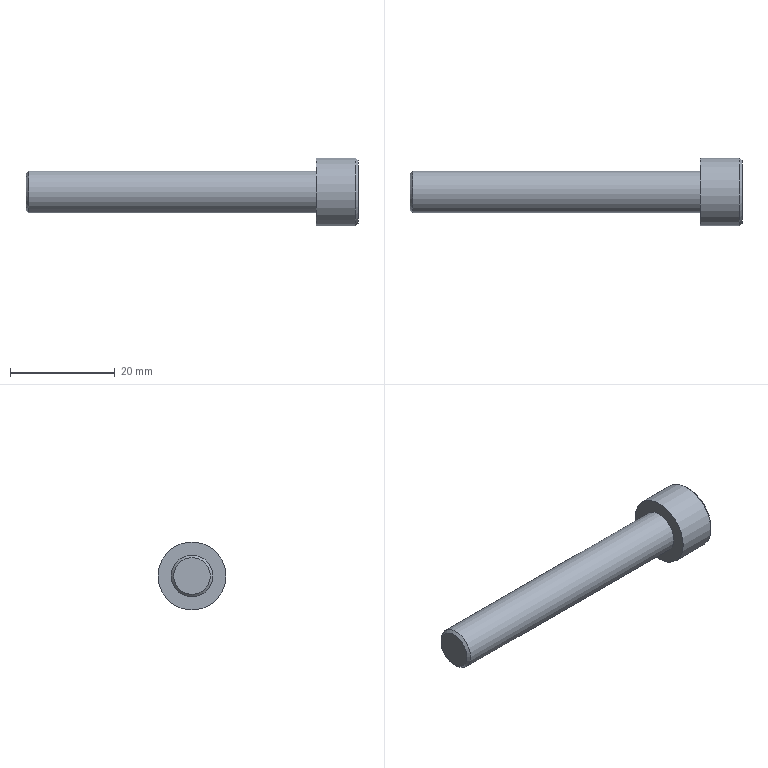Part | NX | features CHAMFER 6, BREP 2, solid 2, SUBTRACT 1 | 1 solid | 36 faces | box 63.5 x 13 x 13 mm | volume 3707 mm3 | plane 23 | spline 9 | cylinder 2 | cone 2 | commonest cylinder face diameters 8 x1 13 x1
STEP:
#1=CARTESIAN_POINT('',(272.5,-202.45,31.002));
#2=VERTEX_POINT('',#1);
#3=CARTESIAN_POINT('',(272.5,-202.625,31.545));
#4=VERTEX_POINT('',#3);
#5=CARTESIAN_POINT('',(272.5,-202.45,31.002));
#6=CARTESIAN_POINT('',(272.5,-202.385,31.002));
#7=CARTESIAN_POINT('',(272.5,-202.327,31.016));
#8=CARTESIAN_POINT('',(272.5,-202.225,31.073));
#9=CARTESIAN_POINT('',(272.5,-202.185,31.113));
#10=CARTESIAN_POINT('',(272.5,-202.128,31.215));
#11=CARTESIAN_POINT('',(272.5,-202.114,31.272));
#12=CARTESIAN_POINT('',(272.5,-202.114,31.377));
#13=CARTESIAN_POINT('',(272.5,-202.121,31.418));
#14=CARTESIAN_POINT('',(272.5,-202.15,31.497));
#15=CARTESIAN_POINT('',(272.5,-202.171,31.531));
#16=CARTESIAN_POINT('',(272.5,-202.224,31.589));
#17=CARTESIAN_POINT('',(272.5,-202.256,31.611));
#18=CARTESIAN_POINT('',(272.5,-202.327,31.643));
#19=CARTESIAN_POINT('',(272.5,-202.366,31.651));
#20=CARTESIAN_POINT('',(272.5,-202.452,31.651));
#21=CARTESIAN_POINT('',(272.5,-202.491,31.642));
#22=CARTESIAN_POINT('',(272.5,-202.562,31.608));
#23=CARTESIAN_POINT('',(272.5,-202.595,31.581));
#24=CARTESIAN_POINT('',(272.5,-202.625,31.545));
#25=B_SPLINE_CURVE_WITH_KNOTS('',3,(#5,#6,#7,#8,#9,#10,#11,#12,#13,#14,#15,#16,#17,#18,#19,#20,#21,#22,#23,#24),.UNSPECIFIED.,.F.,.F.,(4,2,2,2,2,2,2,2,2,4),(0.,0.02844,0.05688,0.08532,0.1049,0.1245,0.144,0.1636,0.184,0.2044),.UNSPECIFIED.);
#26=EDGE_CURVE('',#2,#4,#25,.T.);
#27=ORIENTED_EDGE('',*,*,#26,.F.);
#28=CARTESIAN_POINT('',(272.5,-202.314,31.783));
#29=VERTEX_POINT('',#28);
#30=CARTESIAN_POINT('',(272.5,-202.314,31.783));
#31=CARTESIAN_POINT('',(272.5,-202.306,31.762));
#32=CARTESIAN_POINT('',(272.5,-202.294,31.746));
#33=CARTESIAN_POINT('',(272.5,-202.262,31.722));
#34=CARTESIAN_POINT('',(272.5,-202.245,31.716));
#35=CARTESIAN_POINT('',(272.5,-202.205,31.716));
#36=CARTESIAN_POINT('',(272.5,-202.188,31.724));
#37=CARTESIAN_POINT('',(272.5,-202.16,31.754));
#38=CARTESIAN_POINT('',(272.5,-202.154,31.77));
#39=CARTESIAN_POINT('',(272.5,-202.154,31.818));
#40=CARTESIAN_POINT('',(272.5,-202.164,31.85));
#41=CARTESIAN_POINT('',(272.5,-202.208,31.915));
#42=CARTESIAN_POINT('',(272.5,-202.241,31.943));
#43=CARTESIAN_POINT('',(272.5,-202.327,31.987));
#44=CARTESIAN_POINT('',(272.5,-202.377,31.998));
#45=CARTESIAN_POINT('',(272.5,-202.493,31.998));
#46=CARTESIAN_POINT('',(272.5,-202.545,31.987));
#47=CARTESIAN_POINT('',(272.5,-202.637,31.943));
#48=CARTESIAN_POINT('',(272.5,-202.676,31.91));
#49=CARTESIAN_POINT('',(272.5,-202.741,31.823));
#50=CARTESIAN_POINT('',(272.5,-202.766,31.769));
#51=CARTESIAN_POINT('',(272.5,-202.8,31.637));
#52=CARTESIAN_POINT('',(272.5,-202.809,31.562));
#53=CARTESIAN_POINT('',(272.5,-202.809,31.375));
#54=CARTESIAN_POINT('',(272.5,-202.795,31.288));
#55=CARTESIAN_POINT('',(272.5,-202.738,31.146));
#56=CARTESIAN_POINT('',(272.5,-202.696,31.093));
#57=CARTESIAN_POINT('',(272.5,-202.588,31.02));
#58=CARTESIAN_POINT('',(272.5,-202.524,31.002));
#59=CARTESIAN_POINT('',(272.5,-202.45,31.002));
#60=B_SPLINE_CURVE_WITH_KNOTS('',3,(#30,#31,#32,#33,#34,#35,#36,#37,#38,#39,#40,#41,#42,#43,#44,#45,#46,#47,#48,#49,#50,#51,#52,#53,#54,#55,#56,#57,#58,#59),.UNSPECIFIED.,.F.,.F.,(4,2,2,2,2,2,2,2,2,2,2,2,2,2,4),(0.3727,0.3977,0.4227,0.4513,0.4798,0.5272,0.5745,0.6219,0.6711,0.7203,0.7695,0.8188,0.8792,0.9396,1.),.UNSPECIFIED.);
#61=EDGE_CURVE('',#29,#2,#60,.T.);
#62=ORIENTED_EDGE('',*,*,#61,.F.);
#63=CARTESIAN_POINT('',(272.5,-202.568,31.796));
#64=VERTEX_POINT('',#63);
#65=CARTESIAN_POINT('',(272.5,-202.568,31.796));
#66=CARTESIAN_POINT('',(272.5,-202.552,31.819));
#67=CARTESIAN_POINT('',(272.5,-202.532,31.837));
#68=CARTESIAN_POINT('',(272.5,-202.486,31.864));
#69=CARTESIAN_POINT('',(272.5,-202.463,31.871));
#70=CARTESIAN_POINT('',(272.5,-202.41,31.871));
#71=CARTESIAN_POINT('',(272.5,-202.384,31.863));
#72=CARTESIAN_POINT('',(272.5,-202.34,31.831));
#73=CARTESIAN_POINT('',(272.5,-202.324,31.809));
#74=CARTESIAN_POINT('',(272.5,-202.314,31.783));
#75=B_SPLINE_CURVE_WITH_KNOTS('',3,(#65,#66,#67,#68,#69,#70,#71,#72,#73,#74),.UNSPECIFIED.,.F.,.F.,(4,2,2,2,4),(0.2569,0.2827,0.3085,0.3406,0.3727),.UNSPECIFIED.);
#76=EDGE_CURVE('',#64,#29,#75,.T.);
#77=ORIENTED_EDGE('',*,*,#76,.F.);
#78=CARTESIAN_POINT('',(272.5,-202.625,31.545));
#79=CARTESIAN_POINT('',(272.5,-202.619,31.666));
#80=CARTESIAN_POINT('',(272.5,-202.6,31.749));
#81=CARTESIAN_POINT('',(272.5,-202.568,31.796));
#82=B_SPLINE_CURVE_WITH_KNOTS('',3,(#78,#79,#80,#81),.UNSPECIFIED.,.F.,.F.,(4,4),(0.2044,0.2569),.PIECEWISE_BEZIER_KNOTS.);
#83=EDGE_CURVE('',#4,#64,#82,.T.);
#84=ORIENTED_EDGE('',*,*,#83,.F.);
#85=EDGE_LOOP('',(#27,#62,#77,#84));
#86=FACE_BOUND('',#85,.T.);
#87=CARTESIAN_POINT('',(272.5,-204.732,28.5));
#88=VERTEX_POINT('',#87);
#89=CARTESIAN_POINT('',(272.5,-206.464,31.5));
#90=VERTEX_POINT('',#89);
#91=CARTESIAN_POINT('',(272.5,-206.464,31.5));
#92=DIRECTION('',(0.,-0.5,0.866));
#93=VECTOR('',#92,1000.);
#94=LINE('',#91,#93);
#95=EDGE_CURVE('',#88,#90,#94,.T.);
#96=ORIENTED_EDGE('',*,*,#95,.F.);
#97=CARTESIAN_POINT('',(272.5,-201.268,28.5));
#98=VERTEX_POINT('',#97);
#99=CARTESIAN_POINT('',(272.5,-204.732,28.5));
#100=DIRECTION('',(0.,-1.,0.));
#101=VECTOR('',#100,1000.);
#102=LINE('',#99,#101);
#103=EDGE_CURVE('',#98,#88,#102,.T.);
#104=ORIENTED_EDGE('',*,*,#103,.F.);
#105=CARTESIAN_POINT('',(272.5,-199.536,31.5));
#106=VERTEX_POINT('',#105);
#107=CARTESIAN_POINT('',(272.5,-201.268,28.5));
#108=DIRECTION('',(0.,-0.5,-0.866));
#109=VECTOR('',#108,1000.);
#110=LINE('',#107,#109);
#111=EDGE_CURVE('',#106,#98,#110,.T.);
#112=ORIENTED_EDGE('',*,*,#111,.F.);
#113=CARTESIAN_POINT('',(272.5,-201.268,34.5));
#114=VERTEX_POINT('',#113);
#115=CARTESIAN_POINT('',(272.5,-199.536,31.5));
#116=DIRECTION('',(0.,0.5,-0.866));
#117=VECTOR('',#116,1000.);
#118=LINE('',#115,#117);
#119=EDGE_CURVE('',#114,#106,#118,.T.);
#120=ORIENTED_EDGE('',*,*,#119,.F.);
#121=CARTESIAN_POINT('',(272.5,-204.732,34.5));
#122=VERTEX_POINT('',#121);
#123=CARTESIAN_POINT('',(272.5,-201.268,34.5));
#124=DIRECTION('',(0.,1.,0.));
#125=VECTOR('',#124,1000.);
#126=LINE('',#123,#125);
#127=EDGE_CURVE('',#122,#114,#126,.T.);
#128=ORIENTED_EDGE('',*,*,#127,.F.);
#129=CARTESIAN_POINT('',(272.5,-204.732,34.5));
#130=DIRECTION('',(0.,0.5,0.866));
#131=VECTOR('',#130,1000.);
#132=LINE('',#129,#131);
#133=EDGE_CURVE('',#90,#122,#132,.T.);
#134=ORIENTED_EDGE('',*,*,#133,.F.);
#135=EDGE_LOOP('',(#96,#104,#112,#120,#128,#134));
#136=FACE_BOUND('',#135,.T.);
#137=CARTESIAN_POINT('',(272.5,-203.797,31.005));
#138=VERTEX_POINT('',#137);
#139=CARTESIAN_POINT('',(272.5,-203.706,31.783));
#140=VERTEX_POINT('',#139);
#141=CARTESIAN_POINT('',(272.5,-203.797,31.005));
#142=CARTESIAN_POINT('',(272.5,-203.769,31.005));
#143=CARTESIAN_POINT('',(272.5,-203.748,31.014));
#144=CARTESIAN_POINT('',(272.5,-203.715,31.051));
#145=CARTESIAN_POINT('',(272.5,-203.706,31.079));
#146=CARTESIAN_POINT('',(272.5,-203.706,31.338));
#147=CARTESIAN_POINT('',(272.5,-203.706,31.561));
#148=CARTESIAN_POINT('',(272.5,-203.706,31.783));
#149=B_SPLINE_CURVE_WITH_KNOTS('',3,(#141,#142,#143,#144,#145,#146,#147,#148),.UNSPECIFIED.,.F.,.F.,(4,2,2,4),(0.,0.01767,0.03533,0.1418),.UNSPECIFIED.);
#150=EDGE_CURVE('',#138,#140,#149,.T.);
#151=ORIENTED_EDGE('',*,*,#150,.F.);
#152=CARTESIAN_POINT('',(272.5,-203.561,31.859));
#153=VERTEX_POINT('',#152);
#154=CARTESIAN_POINT('',(272.5,-203.561,31.859));
#155=CARTESIAN_POINT('',(272.5,-203.571,31.898));
#156=CARTESIAN_POINT('',(272.5,-203.58,31.925));
#157=CARTESIAN_POINT('',(272.5,-203.596,31.96));
#158=CARTESIAN_POINT('',(272.5,-203.608,31.972));
#159=CARTESIAN_POINT('',(272.5,-203.641,31.985));
#160=CARTESIAN_POINT('',(272.5,-203.667,31.988));
#161=CARTESIAN_POINT('',(272.5,-203.724,31.988));
#162=CARTESIAN_POINT('',(272.5,-203.744,31.988));
#163=CARTESIAN_POINT('',(272.5,-203.802,31.988));
#164=CARTESIAN_POINT('',(272.5,-203.831,31.981));
#165=CARTESIAN_POINT('',(272.5,-203.875,31.951));
#166=CARTESIAN_POINT('',(272.5,-203.886,31.923));
#167=CARTESIAN_POINT('',(272.5,-203.886,31.626));
#168=CARTESIAN_POINT('',(272.5,-203.886,31.371));
#169=CARTESIAN_POINT('',(272.5,-203.886,31.079));
#170=CARTESIAN_POINT('',(272.5,-203.878,31.051));
#171=CARTESIAN_POINT('',(272.5,-203.845,31.014));
#172=CARTESIAN_POINT('',(272.5,-203.823,31.005));
#173=CARTESIAN_POINT('',(272.5,-203.797,31.005));
#174=B_SPLINE_CURVE_WITH_KNOTS('',3,(#154,#155,#156,#157,#158,#159,#160,#161,#162,#163,#164,#165,#166,#167,#168,#169,#170,#171,#172,#173),.UNSPECIFIED.,.F.,.F.,(4,2,2,2,2,2,2,2,2,4),(0.8075,0.8217,0.8358,0.85,0.8578,0.8723,0.8868,0.9743,0.9872,1.),.UNSPECIFIED.);
#175=EDGE_CURVE('',#153,#138,#174,.T.);
#176=ORIENTED_EDGE('',*,*,#175,.F.);
#177=CARTESIAN_POINT('',(272.5,-203.42,31.33));
#178=VERTEX_POINT('',#177);
#179=CARTESIAN_POINT('',(272.5,-203.435,31.385));
#180=DIRECTION('',(0.,-0.2564,0.9666));
#181=VECTOR('',#180,1000.);
#182=LINE('',#179,#181);
#183=EDGE_CURVE('',#178,#153,#182,.T.);
#184=ORIENTED_EDGE('',*,*,#183,.F.);
#185=CARTESIAN_POINT('',(272.5,-203.28,31.859));
#186=VERTEX_POINT('',#185);
#187=CARTESIAN_POINT('',(272.5,-203.35,31.593));
#188=DIRECTION('',(0.,-0.2564,-0.9666));
#189=VECTOR('',#188,1000.);
#190=LINE('',#187,#189);
#191=EDGE_CURVE('',#186,#178,#190,.T.);
#192=ORIENTED_EDGE('',*,*,#191,.F.);
#193=CARTESIAN_POINT('',(272.5,-203.134,31.783));
#194=VERTEX_POINT('',#193);
#195=CARTESIAN_POINT('',(272.5,-203.134,31.783));
#196=CARTESIAN_POINT('',(272.5,-203.134,31.561));
#197=CARTESIAN_POINT('',(272.5,-203.134,31.338));
#198=CARTESIAN_POINT('',(272.5,-203.134,31.079));
#199=CARTESIAN_POINT('',(272.5,-203.126,31.051));
#200=CARTESIAN_POINT('',(272.5,-203.092,31.014));
#201=CARTESIAN_POINT('',(272.5,-203.071,31.005));
#202=CARTESIAN_POINT('',(272.5,-203.018,31.005));
#203=CARTESIAN_POINT('',(272.5,-202.995,31.014));
#204=CARTESIAN_POINT('',(272.5,-202.962,31.051));
#205=CARTESIAN_POINT('',(272.5,-202.954,31.079));
#206=CARTESIAN_POINT('',(272.5,-202.954,31.371));
#207=CARTESIAN_POINT('',(272.5,-202.954,31.626));
#208=CARTESIAN_POINT('',(272.5,-202.954,31.923));
#209=CARTESIAN_POINT('',(272.5,-202.965,31.951));
#210=CARTESIAN_POINT('',(272.5,-203.009,31.981));
#211=CARTESIAN_POINT('',(272.5,-203.039,31.988));
#212=CARTESIAN_POINT('',(272.5,-203.096,31.988));
#213=CARTESIAN_POINT('',(272.5,-203.117,31.988));
#214=CARTESIAN_POINT('',(272.5,-203.173,31.988));
#215=CARTESIAN_POINT('',(272.5,-203.2,31.985));
#216=CARTESIAN_POINT('',(272.5,-203.233,31.972));
#217=CARTESIAN_POINT('',(272.5,-203.245,31.96));
#218=CARTESIAN_POINT('',(272.5,-203.261,31.925));
#219=CARTESIAN_POINT('',(272.5,-203.27,31.898));
#220=CARTESIAN_POINT('',(272.5,-203.28,31.859));
#221=B_SPLINE_CURVE_WITH_KNOTS('',3,(#195,#196,#197,#198,#199,#200,#201,#202,#203,#204,#205,#206,#207,#208,#209,#210,#211,#212,#213,#214,#215,#216,#217,#218,#219,#220),.UNSPECIFIED.,.F.,.F.,(4,2,2,2,2,2,2,2,2,2,2,2,4),(0.3909,0.4624,0.4743,0.4862,0.4988,0.5115,0.599,0.6135,0.628,0.6359,0.65,0.6642,0.6783),.UNSPECIFIED.);
#222=EDGE_CURVE('',#194,#186,#221,.T.);
#223=ORIENTED_EDGE('',*,*,#222,.F.);
#224=CARTESIAN_POINT('',(272.5,-203.289,31.167));
#225=VERTEX_POINT('',#224);
#226=CARTESIAN_POINT('',(272.5,-203.193,31.549));
#227=DIRECTION('',(0.,0.244,0.9698));
#228=VECTOR('',#227,1000.);
#229=LINE('',#226,#228);
#230=EDGE_CURVE('',#225,#194,#229,.T.);
#231=ORIENTED_EDGE('',*,*,#230,.F.);
#232=CARTESIAN_POINT('',(272.5,-203.551,31.167));
#233=VERTEX_POINT('',#232);
#234=CARTESIAN_POINT('',(272.5,-203.551,31.167));
#235=CARTESIAN_POINT('',(272.5,-203.546,31.147));
#236=CARTESIAN_POINT('',(272.5,-203.541,31.128));
#237=CARTESIAN_POINT('',(272.5,-203.531,31.09));
#238=CARTESIAN_POINT('',(272.5,-203.524,31.073));
#239=CARTESIAN_POINT('',(272.5,-203.506,31.043));
#240=CARTESIAN_POINT('',(272.5,-203.494,31.03));
#241=CARTESIAN_POINT('',(272.5,-203.462,31.01));
#242=CARTESIAN_POINT('',(272.5,-203.443,31.005));
#243=CARTESIAN_POINT('',(272.5,-203.39,31.005));
#244=CARTESIAN_POINT('',(272.5,-203.366,31.013));
#245=CARTESIAN_POINT('',(272.5,-203.332,31.044));
#246=CARTESIAN_POINT('',(272.5,-203.32,31.061));
#247=CARTESIAN_POINT('',(272.5,-203.307,31.098));
#248=CARTESIAN_POINT('',(272.5,-203.299,31.127));
#249=CARTESIAN_POINT('',(272.5,-203.289,31.167));
#250=B_SPLINE_CURVE_WITH_KNOTS('',3,(#234,#235,#236,#237,#238,#239,#240,#241,#242,#243,#244,#245,#246,#247,#248,#249),.UNSPECIFIED.,.F.,.F.,(4,2,2,2,2,2,2,4),(0.243,0.253,0.263,0.273,0.283,0.2963,0.3096,0.3228),.UNSPECIFIED.);
#251=EDGE_CURVE('',#233,#225,#250,.T.);
#252=ORIENTED_EDGE('',*,*,#251,.F.);
#253=CARTESIAN_POINT('',(272.5,-203.597,31.35));
#254=DIRECTION('',(0.,0.244,-0.9698));
#255=VECTOR('',#254,1000.);
#256=LINE('',#253,#255);
#257=EDGE_CURVE('',#140,#233,#256,.T.);
#258=ORIENTED_EDGE('',*,*,#257,.F.);
#259=EDGE_LOOP('',(#151,#176,#184,#192,#223,#231,#252,#258));
#260=FACE_BOUND('',#259,.T.);
#261=CARTESIAN_POINT('',(272.5,-203.,31.5));
#262=DIRECTION('',(1.,0.,0.));
#263=DIRECTION('',(0.,-1.,0.));
#264=AXIS2_PLACEMENT_3D('',#261,#262,#263);
#265=PLANE('',#264);
#266=ADVANCED_FACE('',(#86,#136,#260),#265,.T.);
#267=CARTESIAN_POINT('',(213.,-206.5,31.5));
#268=VERTEX_POINT('',#267);
#269=CARTESIAN_POINT('',(213.,-203.,31.5));
#270=DIRECTION('',(-1.,0.,0.));
#271=DIRECTION('',(0.,-1.,0.));
#272=AXIS2_PLACEMENT_3D('',#269,#270,#271);
#273=CIRCLE('',#272,3.5);
#274=EDGE_CURVE('',#268,#268,#273,.T.);
#275=ORIENTED_EDGE('',*,*,#274,.T.);
#276=EDGE_LOOP('',(#275));
#277=FACE_BOUND('',#276,.T.);
#278=CARTESIAN_POINT('',(213.,-203.,27.5));
#279=DIRECTION('',(-1.,0.,0.));
#280=DIRECTION('',(0.,1.,0.));
#281=AXIS2_PLACEMENT_3D('',#278,#279,#280);
#282=PLANE('',#281);
#283=ADVANCED_FACE('',(#277),#282,.T.);
#284=CARTESIAN_POINT('',(213.5,-207.,31.5));
#285=VERTEX_POINT('',#284);
#286=CARTESIAN_POINT('',(213.5,-203.,31.5));
#287=DIRECTION('',(1.,0.,0.));
#288=DIRECTION('',(0.,-1.,0.));
#289=AXIS2_PLACEMENT_3D('',#286,#287,#288);
#290=CIRCLE('',#289,4.);
#291=EDGE_CURVE('',#285,#285,#290,.T.);
#292=ORIENTED_EDGE('',*,*,#291,.T.);
#293=EDGE_LOOP('',(#292));
#294=FACE_BOUND('',#293,.T.);
#295=CARTESIAN_POINT('',(268.5,-199.,31.5));
#296=VERTEX_POINT('',#295);
#297=CARTESIAN_POINT('',(268.5,-203.,31.5));
#298=DIRECTION('',(1.,0.,0.));
#299=DIRECTION('',(0.,1.,0.));
#300=AXIS2_PLACEMENT_3D('',#297,#298,#299);
#301=CIRCLE('',#300,4.);
#302=EDGE_CURVE('',#296,#296,#301,.T.);
#303=ORIENTED_EDGE('',*,*,#302,.F.);
#304=EDGE_LOOP('',(#303));
#305=FACE_BOUND('',#304,.T.);
#306=CARTESIAN_POINT('',(277.5,-203.,31.5));
#307=DIRECTION('',(1.,0.,0.));
#308=DIRECTION('',(0.,-1.,0.));
#309=AXIS2_PLACEMENT_3D('',#306,#307,#308);
#310=CYLINDRICAL_SURFACE('',#309,4.);
#311=ADVANCED_FACE('',(#294,#305),#310,.T.);
#312=ORIENTED_EDGE('',*,*,#302,.T.);
#313=EDGE_LOOP('',(#312));
#314=FACE_BOUND('',#313,.T.);
#315=CARTESIAN_POINT('',(268.5,-196.5,31.5));
#316=VERTEX_POINT('',#315);
#317=CARTESIAN_POINT('',(268.5,-203.,31.5));
#318=DIRECTION('',(1.,0.,0.));
#319=DIRECTION('',(0.,1.,0.));
#320=AXIS2_PLACEMENT_3D('',#317,#318,#319);
#321=CIRCLE('',#320,6.5);
#322=EDGE_CURVE('',#316,#316,#321,.T.);
#323=ORIENTED_EDGE('',*,*,#322,.F.);
#324=EDGE_LOOP('',(#323));
#325=FACE_BOUND('',#324,.T.);
#326=CARTESIAN_POINT('',(268.5,-203.,25.));
#327=DIRECTION('',(-1.,0.,0.));
#328=DIRECTION('',(0.,1.,0.));
#329=AXIS2_PLACEMENT_3D('',#326,#327,#328);
#330=PLANE('',#329);
#331=ADVANCED_FACE('',(#314,#325),#330,.T.);
#332=CARTESIAN_POINT('',(276.,-196.5,31.5));
#333=VERTEX_POINT('',#332);
#334=CARTESIAN_POINT('',(276.,-203.,31.5));
#335=DIRECTION('',(-1.,0.,0.));
#336=DIRECTION('',(0.,1.,0.));
#337=AXIS2_PLACEMENT_3D('',#334,#335,#336);
#338=CIRCLE('',#337,6.5);
#339=EDGE_CURVE('',#333,#333,#338,.T.);
#340=ORIENTED_EDGE('',*,*,#339,.T.);
#341=EDGE_LOOP('',(#340));
#342=FACE_BOUND('',#341,.T.);
#343=ORIENTED_EDGE('',*,*,#322,.T.);
#344=EDGE_LOOP('',(#343));
#345=FACE_BOUND('',#344,.T.);
#346=CARTESIAN_POINT('',(277.5,-203.,31.5));
#347=DIRECTION('',(1.,0.,0.));
#348=DIRECTION('',(0.,-1.,0.));
#349=AXIS2_PLACEMENT_3D('',#346,#347,#348);
#350=CYLINDRICAL_SURFACE('',#349,6.5);
#351=ADVANCED_FACE('',(#342,#345),#350,.T.);
#352=CARTESIAN_POINT('',(276.5,-197.,31.5));
#353=VERTEX_POINT('',#352);
#354=CARTESIAN_POINT('',(276.5,-203.,31.5));
#355=DIRECTION('',(1.,0.,0.));
#356=DIRECTION('',(0.,1.,0.));
#357=AXIS2_PLACEMENT_3D('',#354,#355,#356);
#358=CIRCLE('',#357,6.);
#359=EDGE_CURVE('',#353,#353,#358,.T.);
#360=ORIENTED_EDGE('',*,*,#359,.T.);
#361=EDGE_LOOP('',(#360));
#362=FACE_BOUND('',#361,.T.);
#363=CARTESIAN_POINT('',(276.5,-205.309,27.5));
#364=VERTEX_POINT('',#363);
#365=CARTESIAN_POINT('',(276.5,-207.619,31.5));
#366=VERTEX_POINT('',#365);
#367=CARTESIAN_POINT('',(276.5,-207.33,31.));
#368=DIRECTION('',(0.,-0.5,0.866));
#369=VECTOR('',#368,1000.);
#370=LINE('',#367,#369);
#371=EDGE_CURVE('',#364,#366,#370,.T.);
#372=ORIENTED_EDGE('',*,*,#371,.T.);
#373=CARTESIAN_POINT('',(276.5,-205.309,35.5));
#374=VERTEX_POINT('',#373);
#375=CARTESIAN_POINT('',(276.5,-205.021,36.));
#376=DIRECTION('',(0.,0.5,0.866));
#377=VECTOR('',#376,1000.);
#378=LINE('',#375,#377);
#379=EDGE_CURVE('',#366,#374,#378,.T.);
#380=ORIENTED_EDGE('',*,*,#379,.T.);
#381=CARTESIAN_POINT('',(276.5,-200.691,35.5));
#382=VERTEX_POINT('',#381);
#383=CARTESIAN_POINT('',(276.5,-200.113,35.5));
#384=DIRECTION('',(0.,1.,0.));
#385=VECTOR('',#384,1000.);
#386=LINE('',#383,#385);
#387=EDGE_CURVE('',#374,#382,#386,.T.);
#388=ORIENTED_EDGE('',*,*,#387,.T.);
#389=CARTESIAN_POINT('',(276.5,-198.381,31.5));
#390=VERTEX_POINT('',#389);
#391=CARTESIAN_POINT('',(276.5,-198.093,31.));
#392=DIRECTION('',(0.,0.5,-0.866));
#393=VECTOR('',#392,1000.);
#394=LINE('',#391,#393);
#395=EDGE_CURVE('',#382,#390,#394,.T.);
#396=ORIENTED_EDGE('',*,*,#395,.T.);
#397=CARTESIAN_POINT('',(276.5,-200.691,27.5));
#398=VERTEX_POINT('',#397);
#399=CARTESIAN_POINT('',(276.5,-200.979,27.));
#400=DIRECTION('',(0.,-0.5,-0.866));
#401=VECTOR('',#400,1000.);
#402=LINE('',#399,#401);
#403=EDGE_CURVE('',#390,#398,#402,.T.);
#404=ORIENTED_EDGE('',*,*,#403,.T.);
#405=CARTESIAN_POINT('',(276.5,-205.887,27.5));
#406=DIRECTION('',(0.,-1.,0.));
#407=VECTOR('',#406,1000.);
#408=LINE('',#405,#407);
#409=EDGE_CURVE('',#398,#364,#408,.T.);
#410=ORIENTED_EDGE('',*,*,#409,.T.);
#411=EDGE_LOOP('',(#372,#380,#388,#396,#404,#410));
#412=FACE_BOUND('',#411,.T.);
#413=CARTESIAN_POINT('',(276.5,-203.,31.5));
#414=DIRECTION('',(1.,0.,0.));
#415=DIRECTION('',(0.,-1.,0.));
#416=AXIS2_PLACEMENT_3D('',#413,#414,#415);
#417=PLANE('',#416);
#418=ADVANCED_FACE('',(#362,#412),#417,.T.);
#419=CARTESIAN_POINT('',(275.5,-206.464,31.5));
#420=VERTEX_POINT('',#419);
#421=CARTESIAN_POINT('',(272.5,-206.464,31.5));
#422=DIRECTION('',(-1.,0.,0.));
#423=VECTOR('',#422,1000.);
#424=LINE('',#421,#423);
#425=EDGE_CURVE('',#420,#90,#424,.T.);
#426=ORIENTED_EDGE('',*,*,#425,.F.);
#427=CARTESIAN_POINT('',(275.5,-204.732,28.5));
#428=VERTEX_POINT('',#427);
#429=CARTESIAN_POINT('',(275.5,-204.732,28.5));
#430=DIRECTION('',(0.,0.5,-0.866));
#431=VECTOR('',#430,1000.);
#432=LINE('',#429,#431);
#433=EDGE_CURVE('',#420,#428,#432,.T.);
#434=ORIENTED_EDGE('',*,*,#433,.T.);
#435=CARTESIAN_POINT('',(272.5,-204.732,28.5));
#436=DIRECTION('',(-1.,0.,0.));
#437=VECTOR('',#436,1000.);
#438=LINE('',#435,#437);
#439=EDGE_CURVE('',#428,#88,#438,.T.);
#440=ORIENTED_EDGE('',*,*,#439,.T.);
#441=ORIENTED_EDGE('',*,*,#95,.T.);
#442=EDGE_LOOP('',(#426,#434,#440,#441));
#443=FACE_BOUND('',#442,.T.);
#444=CARTESIAN_POINT('',(272.5,-206.464,31.5));
#445=DIRECTION('',(0.,-0.866,-0.5));
#446=DIRECTION('',(0.,-0.5,0.866));
#447=AXIS2_PLACEMENT_3D('',#444,#445,#446);
#448=PLANE('',#447);
#449=ADVANCED_FACE('',(#443),#448,.F.);
#450=ORIENTED_EDGE('',*,*,#439,.F.);
#451=CARTESIAN_POINT('',(275.5,-201.268,28.5));
#452=VERTEX_POINT('',#451);
#453=CARTESIAN_POINT('',(275.5,-201.268,28.5));
#454=DIRECTION('',(0.,1.,0.));
#455=VECTOR('',#454,1000.);
#456=LINE('',#453,#455);
#457=EDGE_CURVE('',#428,#452,#456,.T.);
#458=ORIENTED_EDGE('',*,*,#457,.T.);
#459=CARTESIAN_POINT('',(272.5,-201.268,28.5));
#460=DIRECTION('',(-1.,0.,0.));
#461=VECTOR('',#460,1000.);
#462=LINE('',#459,#461);
#463=EDGE_CURVE('',#452,#98,#462,.T.);
#464=ORIENTED_EDGE('',*,*,#463,.T.);
#465=ORIENTED_EDGE('',*,*,#103,.T.);
#466=EDGE_LOOP('',(#450,#458,#464,#465));
#467=FACE_BOUND('',#466,.T.);
#468=CARTESIAN_POINT('',(272.5,-204.732,28.5));
#469=DIRECTION('',(0.,0.,-1.));
#470=DIRECTION('',(0.,-1.,0.));
#471=AXIS2_PLACEMENT_3D('',#468,#469,#470);
#472=PLANE('',#471);
#473=ADVANCED_FACE('',(#467),#472,.F.);
#474=ORIENTED_EDGE('',*,*,#463,.F.);
#475=CARTESIAN_POINT('',(275.5,-199.536,31.5));
#476=VERTEX_POINT('',#475);
#477=CARTESIAN_POINT('',(275.5,-199.536,31.5));
#478=DIRECTION('',(0.,0.5,0.866));
#479=VECTOR('',#478,1000.);
#480=LINE('',#477,#479);
#481=EDGE_CURVE('',#452,#476,#480,.T.);
#482=ORIENTED_EDGE('',*,*,#481,.T.);
#483=CARTESIAN_POINT('',(272.5,-199.536,31.5));
#484=DIRECTION('',(-1.,0.,0.));
#485=VECTOR('',#484,1000.);
#486=LINE('',#483,#485);
#487=EDGE_CURVE('',#476,#106,#486,.T.);
#488=ORIENTED_EDGE('',*,*,#487,.T.);
#489=ORIENTED_EDGE('',*,*,#111,.T.);
#490=EDGE_LOOP('',(#474,#482,#488,#489));
#491=FACE_BOUND('',#490,.T.);
#492=CARTESIAN_POINT('',(272.5,-201.268,28.5));
#493=DIRECTION('',(0.,0.866,-0.5));
#494=DIRECTION('',(0.,-0.5,-0.866));
#495=AXIS2_PLACEMENT_3D('',#492,#493,#494);
#496=PLANE('',#495);
#497=ADVANCED_FACE('',(#491),#496,.F.);
#498=ORIENTED_EDGE('',*,*,#487,.F.);
#499=CARTESIAN_POINT('',(275.5,-201.268,34.5));
#500=VERTEX_POINT('',#499);
#501=CARTESIAN_POINT('',(275.5,-201.268,34.5));
#502=DIRECTION('',(0.,-0.5,0.866));
#503=VECTOR('',#502,1000.);
#504=LINE('',#501,#503);
#505=EDGE_CURVE('',#476,#500,#504,.T.);
#506=ORIENTED_EDGE('',*,*,#505,.T.);
#507=CARTESIAN_POINT('',(272.5,-201.268,34.5));
#508=DIRECTION('',(-1.,0.,0.));
#509=VECTOR('',#508,1000.);
#510=LINE('',#507,#509);
#511=EDGE_CURVE('',#500,#114,#510,.T.);
#512=ORIENTED_EDGE('',*,*,#511,.T.);
#513=ORIENTED_EDGE('',*,*,#119,.T.);
#514=EDGE_LOOP('',(#498,#506,#512,#513));
#515=FACE_BOUND('',#514,.T.);
#516=CARTESIAN_POINT('',(272.5,-199.536,31.5));
#517=DIRECTION('',(0.,0.866,0.5));
#518=DIRECTION('',(0.,0.5,-0.866));
#519=AXIS2_PLACEMENT_3D('',#516,#517,#518);
#520=PLANE('',#519);
#521=ADVANCED_FACE('',(#515),#520,.F.);
#522=ORIENTED_EDGE('',*,*,#511,.F.);
#523=CARTESIAN_POINT('',(275.5,-204.732,34.5));
#524=VERTEX_POINT('',#523);
#525=CARTESIAN_POINT('',(275.5,-204.732,34.5));
#526=DIRECTION('',(0.,-1.,0.));
#527=VECTOR('',#526,1000.);
#528=LINE('',#525,#527);
#529=EDGE_CURVE('',#500,#524,#528,.T.);
#530=ORIENTED_EDGE('',*,*,#529,.T.);
#531=CARTESIAN_POINT('',(272.5,-204.732,34.5));
#532=DIRECTION('',(-1.,0.,0.));
#533=VECTOR('',#532,1000.);
#534=LINE('',#531,#533);
#535=EDGE_CURVE('',#524,#122,#534,.T.);
#536=ORIENTED_EDGE('',*,*,#535,.T.);
#537=ORIENTED_EDGE('',*,*,#127,.T.);
#538=EDGE_LOOP('',(#522,#530,#536,#537));
#539=FACE_BOUND('',#538,.T.);
#540=CARTESIAN_POINT('',(272.5,-201.268,34.5));
#541=DIRECTION('',(0.,0.,1.));
#542=DIRECTION('',(-1.,0.,0.));
#543=AXIS2_PLACEMENT_3D('',#540,#541,#542);
#544=PLANE('',#543);
#545=ADVANCED_FACE('',(#539),#544,.F.);
#546=ORIENTED_EDGE('',*,*,#535,.F.);
#547=CARTESIAN_POINT('',(275.5,-207.041,30.5));
#548=DIRECTION('',(0.,-0.5,-0.866));
#549=VECTOR('',#548,1000.);
#550=LINE('',#547,#549);
#551=EDGE_CURVE('',#524,#420,#550,.T.);
#552=ORIENTED_EDGE('',*,*,#551,.T.);
#553=ORIENTED_EDGE('',*,*,#425,.T.);
#554=ORIENTED_EDGE('',*,*,#133,.T.);
#555=EDGE_LOOP('',(#546,#552,#553,#554));
#556=FACE_BOUND('',#555,.T.);
#557=CARTESIAN_POINT('',(272.5,-204.732,34.5));
#558=DIRECTION('',(0.,-0.866,0.5));
#559=DIRECTION('',(0.,0.5,0.866));
#560=AXIS2_PLACEMENT_3D('',#557,#558,#559);
#561=PLANE('',#560);
#562=ADVANCED_FACE('',(#556),#561,.F.);
#563=ORIENTED_EDGE('',*,*,#274,.F.);
#564=EDGE_LOOP('',(#563));
#565=FACE_BOUND('',#564,.T.);
#566=ORIENTED_EDGE('',*,*,#291,.F.);
#567=EDGE_LOOP('',(#566));
#568=FACE_BOUND('',#567,.T.);
#569=CARTESIAN_POINT('',(213.5,-203.,31.5));
#570=DIRECTION('',(1.,0.,0.));
#571=DIRECTION('',(0.,-1.,0.));
#572=AXIS2_PLACEMENT_3D('',#569,#570,#571);
#573=CONICAL_SURFACE('',#572,4.,0.7854);
#574=ADVANCED_FACE('',(#565,#568),#573,.T.);
#575=ORIENTED_EDGE('',*,*,#339,.F.);
#576=EDGE_LOOP('',(#575));
#577=FACE_BOUND('',#576,.T.);
#578=ORIENTED_EDGE('',*,*,#359,.F.);
#579=EDGE_LOOP('',(#578));
#580=FACE_BOUND('',#579,.T.);
#581=CARTESIAN_POINT('',(276.5,-203.,31.5));
#582=DIRECTION('',(-1.,0.,0.));
#583=DIRECTION('',(0.,1.,0.));
#584=AXIS2_PLACEMENT_3D('',#581,#582,#583);
#585=CONICAL_SURFACE('',#584,6.,0.7854);
#586=ADVANCED_FACE('',(#577,#580),#585,.T.);
#587=ORIENTED_EDGE('',*,*,#150,.T.);
#588=CARTESIAN_POINT('',(272.3,-203.706,31.783));
#589=VERTEX_POINT('',#588);
#590=CARTESIAN_POINT('',(272.3,-203.706,31.783));
#591=DIRECTION('',(1.,0.,0.));
#592=VECTOR('',#591,1000.);
#593=LINE('',#590,#592);
#594=EDGE_CURVE('',#140,#589,#593,.F.);
#595=ORIENTED_EDGE('',*,*,#594,.T.);
#596=CARTESIAN_POINT('',(272.3,-203.797,31.005));
#597=VERTEX_POINT('',#596);
#598=CARTESIAN_POINT('',(272.3,-203.797,31.005));
#599=CARTESIAN_POINT('',(272.3,-203.769,31.005));
#600=CARTESIAN_POINT('',(272.3,-203.748,31.014));
#601=CARTESIAN_POINT('',(272.3,-203.715,31.051));
#602=CARTESIAN_POINT('',(272.3,-203.706,31.079));
#603=CARTESIAN_POINT('',(272.3,-203.706,31.338));
#604=CARTESIAN_POINT('',(272.3,-203.706,31.561));
#605=CARTESIAN_POINT('',(272.3,-203.706,31.783));
#606=B_SPLINE_CURVE_WITH_KNOTS('',3,(#598,#599,#600,#601,#602,#603,#604,#605),.UNSPECIFIED.,.F.,.F.,(4,2,2,4),(0.,0.01767,0.03533,0.1418),.UNSPECIFIED.);
#607=EDGE_CURVE('',#589,#597,#606,.F.);
#608=ORIENTED_EDGE('',*,*,#607,.T.);
#609=CARTESIAN_POINT('',(272.3,-203.797,31.005));
#610=DIRECTION('',(1.,0.,0.));
#611=VECTOR('',#610,1000.);
#612=LINE('',#609,#611);
#613=EDGE_CURVE('',#138,#597,#612,.F.);
#614=ORIENTED_EDGE('',*,*,#613,.F.);
#615=EDGE_LOOP('',(#587,#595,#608,#614));
#616=FACE_BOUND('',#615,.T.);
#617=CARTESIAN_POINT('',(272.3,-203.797,31.005));
#618=CARTESIAN_POINT('',(272.5,-203.797,31.005));
#619=CARTESIAN_POINT('',(272.3,-203.687,31.005));
#620=CARTESIAN_POINT('',(272.5,-203.687,31.005));
#621=CARTESIAN_POINT('',(272.3,-203.716,31.357));
#622=CARTESIAN_POINT('',(272.5,-203.716,31.357));
#623=CARTESIAN_POINT('',(272.3,-203.706,31.635));
#624=CARTESIAN_POINT('',(272.5,-203.706,31.635));
#625=CARTESIAN_POINT('',(272.3,-203.706,31.783));
#626=CARTESIAN_POINT('',(272.5,-203.706,31.783));
#627=B_SPLINE_SURFACE_WITH_KNOTS('',3,1,((#617,#618),(#619,#620),(#621,#622),(#623,#624),(#625,#626)),.SURF_OF_LINEAR_EXTRUSION.,.F.,.F.,.F.,(4,1,4),(2,2),(0.,0.07088,0.1418),(0.,1.),.UNSPECIFIED.);
#628=ADVANCED_FACE('',(#616),#627,.F.);
#629=ORIENTED_EDGE('',*,*,#257,.T.);
#630=CARTESIAN_POINT('',(272.3,-203.551,31.167));
#631=VERTEX_POINT('',#630);
#632=CARTESIAN_POINT('',(272.3,-203.551,31.167));
#633=DIRECTION('',(1.,0.,0.));
#634=VECTOR('',#633,1000.);
#635=LINE('',#632,#634);
#636=EDGE_CURVE('',#233,#631,#635,.F.);
#637=ORIENTED_EDGE('',*,*,#636,.T.);
#638=CARTESIAN_POINT('',(272.3,-203.706,31.783));
#639=CARTESIAN_POINT('',(272.3,-203.655,31.578));
#640=CARTESIAN_POINT('',(272.3,-203.603,31.373));
#641=CARTESIAN_POINT('',(272.3,-203.551,31.167));
#642=B_SPLINE_CURVE_WITH_KNOTS('',3,(#638,#639,#640,#641),.UNSPECIFIED.,.F.,.F.,(4,4),(0.1418,0.243),.PIECEWISE_BEZIER_KNOTS.);
#643=EDGE_CURVE('',#631,#589,#642,.F.);
#644=ORIENTED_EDGE('',*,*,#643,.T.);
#645=ORIENTED_EDGE('',*,*,#594,.F.);
#646=EDGE_LOOP('',(#629,#637,#644,#645));
#647=FACE_BOUND('',#646,.T.);
#648=CARTESIAN_POINT('',(272.3,-203.706,31.783));
#649=DIRECTION('',(0.,-0.9698,-0.244));
#650=DIRECTION('',(0.,0.244,-0.9698));
#651=AXIS2_PLACEMENT_3D('',#648,#649,#650);
#652=PLANE('',#651);
#653=ADVANCED_FACE('',(#647),#652,.F.);
#654=ORIENTED_EDGE('',*,*,#251,.T.);
#655=CARTESIAN_POINT('',(272.3,-203.289,31.167));
#656=VERTEX_POINT('',#655);
#657=CARTESIAN_POINT('',(272.3,-203.289,31.167));
#658=DIRECTION('',(1.,0.,0.));
#659=VECTOR('',#658,1000.);
#660=LINE('',#657,#659);
#661=EDGE_CURVE('',#225,#656,#660,.F.);
#662=ORIENTED_EDGE('',*,*,#661,.T.);
#663=CARTESIAN_POINT('',(272.3,-203.551,31.167));
#664=CARTESIAN_POINT('',(272.3,-203.546,31.147));
#665=CARTESIAN_POINT('',(272.3,-203.541,31.128));
#666=CARTESIAN_POINT('',(272.3,-203.531,31.09));
#667=CARTESIAN_POINT('',(272.3,-203.524,31.073));
#668=CARTESIAN_POINT('',(272.3,-203.506,31.043));
#669=CARTESIAN_POINT('',(272.3,-203.494,31.03));
#670=CARTESIAN_POINT('',(272.3,-203.462,31.01));
#671=CARTESIAN_POINT('',(272.3,-203.443,31.005));
#672=CARTESIAN_POINT('',(272.3,-203.39,31.005));
#673=CARTESIAN_POINT('',(272.3,-203.366,31.013));
#674=CARTESIAN_POINT('',(272.3,-203.332,31.044));
#675=CARTESIAN_POINT('',(272.3,-203.32,31.061));
#676=CARTESIAN_POINT('',(272.3,-203.307,31.098));
#677=CARTESIAN_POINT('',(272.3,-203.299,31.127));
#678=CARTESIAN_POINT('',(272.3,-203.289,31.167));
#679=B_SPLINE_CURVE_WITH_KNOTS('',3,(#663,#664,#665,#666,#667,#668,#669,#670,#671,#672,#673,#674,#675,#676,#677,#678),.UNSPECIFIED.,.F.,.F.,(4,2,2,2,2,2,2,4),(0.243,0.253,0.263,0.273,0.283,0.2963,0.3096,0.3228),.UNSPECIFIED.);
#680=EDGE_CURVE('',#656,#631,#679,.F.);
#681=ORIENTED_EDGE('',*,*,#680,.T.);
#682=ORIENTED_EDGE('',*,*,#636,.F.);
#683=EDGE_LOOP('',(#654,#662,#681,#682));
#684=FACE_BOUND('',#683,.T.);
#685=CARTESIAN_POINT('',(272.3,-203.551,31.167));
#686=CARTESIAN_POINT('',(272.5,-203.551,31.167));
#687=CARTESIAN_POINT('',(272.3,-203.509,31.006));
#688=CARTESIAN_POINT('',(272.5,-203.509,31.006));
#689=CARTESIAN_POINT('',(272.3,-203.35,30.927));
#690=CARTESIAN_POINT('',(272.5,-203.35,30.927));
#691=CARTESIAN_POINT('',(272.3,-203.289,31.167));
#692=CARTESIAN_POINT('',(272.5,-203.289,31.167));
#693=B_SPLINE_SURFACE_WITH_KNOTS('',3,1,((#685,#686),(#687,#688),(#689,#690),(#691,#692)),.SURF_OF_LINEAR_EXTRUSION.,.F.,.F.,.F.,(4,4),(2,2),(0.243,0.3228),(0.,1.),.PIECEWISE_BEZIER_KNOTS.);
#694=ADVANCED_FACE('',(#684),#693,.F.);
#695=ORIENTED_EDGE('',*,*,#230,.T.);
#696=CARTESIAN_POINT('',(272.3,-203.134,31.783));
#697=VERTEX_POINT('',#696);
#698=CARTESIAN_POINT('',(272.3,-203.134,31.783));
#699=DIRECTION('',(1.,0.,0.));
#700=VECTOR('',#699,1000.);
#701=LINE('',#698,#700);
#702=EDGE_CURVE('',#194,#697,#701,.F.);
#703=ORIENTED_EDGE('',*,*,#702,.T.);
#704=CARTESIAN_POINT('',(272.3,-203.289,31.167));
#705=CARTESIAN_POINT('',(272.3,-203.237,31.373));
#706=CARTESIAN_POINT('',(272.3,-203.186,31.578));
#707=CARTESIAN_POINT('',(272.3,-203.134,31.783));
#708=B_SPLINE_CURVE_WITH_KNOTS('',3,(#704,#705,#706,#707),.UNSPECIFIED.,.F.,.F.,(4,4),(0.3228,0.3909),.PIECEWISE_BEZIER_KNOTS.);
#709=EDGE_CURVE('',#697,#656,#708,.F.);
#710=ORIENTED_EDGE('',*,*,#709,.T.);
#711=ORIENTED_EDGE('',*,*,#661,.F.);
#712=EDGE_LOOP('',(#695,#703,#710,#711));
#713=FACE_BOUND('',#712,.T.);
#714=CARTESIAN_POINT('',(272.3,-203.289,31.167));
#715=DIRECTION('',(0.,0.9698,-0.244));
#716=DIRECTION('',(0.,0.244,0.9698));
#717=AXIS2_PLACEMENT_3D('',#714,#715,#716);
#718=PLANE('',#717);
#719=ADVANCED_FACE('',(#713),#718,.F.);
#720=ORIENTED_EDGE('',*,*,#222,.T.);
#721=CARTESIAN_POINT('',(272.3,-203.28,31.859));
#722=VERTEX_POINT('',#721);
#723=CARTESIAN_POINT('',(272.3,-203.28,31.859));
#724=DIRECTION('',(1.,0.,0.));
#725=VECTOR('',#724,1000.);
#726=LINE('',#723,#725);
#727=EDGE_CURVE('',#186,#722,#726,.F.);
#728=ORIENTED_EDGE('',*,*,#727,.T.);
#729=CARTESIAN_POINT('',(272.3,-203.134,31.783));
#730=CARTESIAN_POINT('',(272.3,-203.134,31.561));
#731=CARTESIAN_POINT('',(272.3,-203.134,31.338));
#732=CARTESIAN_POINT('',(272.3,-203.134,31.079));
#733=CARTESIAN_POINT('',(272.3,-203.126,31.051));
#734=CARTESIAN_POINT('',(272.3,-203.092,31.014));
#735=CARTESIAN_POINT('',(272.3,-203.071,31.005));
#736=CARTESIAN_POINT('',(272.3,-203.018,31.005));
#737=CARTESIAN_POINT('',(272.3,-202.995,31.014));
#738=CARTESIAN_POINT('',(272.3,-202.962,31.051));
#739=CARTESIAN_POINT('',(272.3,-202.954,31.079));
#740=CARTESIAN_POINT('',(272.3,-202.954,31.371));
#741=CARTESIAN_POINT('',(272.3,-202.954,31.626));
#742=CARTESIAN_POINT('',(272.3,-202.954,31.923));
#743=CARTESIAN_POINT('',(272.3,-202.965,31.951));
#744=CARTESIAN_POINT('',(272.3,-203.009,31.981));
#745=CARTESIAN_POINT('',(272.3,-203.039,31.988));
#746=CARTESIAN_POINT('',(272.3,-203.096,31.988));
#747=CARTESIAN_POINT('',(272.3,-203.117,31.988));
#748=CARTESIAN_POINT('',(272.3,-203.173,31.988));
#749=CARTESIAN_POINT('',(272.3,-203.2,31.985));
#750=CARTESIAN_POINT('',(272.3,-203.233,31.972));
#751=CARTESIAN_POINT('',(272.3,-203.245,31.96));
#752=CARTESIAN_POINT('',(272.3,-203.261,31.925));
#753=CARTESIAN_POINT('',(272.3,-203.27,31.898));
#754=CARTESIAN_POINT('',(272.3,-203.28,31.859));
#755=B_SPLINE_CURVE_WITH_KNOTS('',3,(#729,#730,#731,#732,#733,#734,#735,#736,#737,#738,#739,#740,#741,#742,#743,#744,#745,#746,#747,#748,#749,#750,#751,#752,#753,#754),.UNSPECIFIED.,.F.,.F.,(4,2,2,2,2,2,2,2,2,2,2,2,4),(0.3909,0.4624,0.4743,0.4862,0.4988,0.5115,0.599,0.6135,0.628,0.6359,0.65,0.6642,0.6783),.UNSPECIFIED.);
#756=EDGE_CURVE('',#722,#697,#755,.F.);
#757=ORIENTED_EDGE('',*,*,#756,.T.);
#758=ORIENTED_EDGE('',*,*,#702,.F.);
#759=EDGE_LOOP('',(#720,#728,#757,#758));
#760=FACE_BOUND('',#759,.T.);
#761=CARTESIAN_POINT('',(272.3,-203.134,31.783));
#762=CARTESIAN_POINT('',(272.5,-203.134,31.783));
#763=CARTESIAN_POINT('',(272.3,-203.134,31.671));
#764=CARTESIAN_POINT('',(272.5,-203.134,31.671));
#765=CARTESIAN_POINT('',(272.3,-203.119,31.461));
#766=CARTESIAN_POINT('',(272.5,-203.119,31.461));
#767=CARTESIAN_POINT('',(272.3,-203.188,31.067));
#768=CARTESIAN_POINT('',(272.5,-203.188,31.067));
#769=CARTESIAN_POINT('',(272.3,-202.933,30.947));
#770=CARTESIAN_POINT('',(272.5,-202.933,30.947));
#771=CARTESIAN_POINT('',(272.3,-202.956,31.336));
#772=CARTESIAN_POINT('',(272.5,-202.956,31.336));
#773=CARTESIAN_POINT('',(272.3,-202.969,31.613));
#774=CARTESIAN_POINT('',(272.5,-202.969,31.613));
#775=CARTESIAN_POINT('',(272.3,-202.894,32.));
#776=CARTESIAN_POINT('',(272.5,-202.894,32.));
#777=CARTESIAN_POINT('',(272.3,-203.231,31.994));
#778=CARTESIAN_POINT('',(272.5,-203.231,31.994));
#779=CARTESIAN_POINT('',(272.3,-203.254,31.957));
#780=CARTESIAN_POINT('',(272.5,-203.254,31.957));
#781=CARTESIAN_POINT('',(272.3,-203.28,31.859));
#782=CARTESIAN_POINT('',(272.5,-203.28,31.859));
#783=B_SPLINE_SURFACE_WITH_KNOTS('',3,1,((#761,#762),(#763,#764),(#765,#766),(#767,#768),(#769,#770),(#771,#772),(#773,#774),(#775,#776),(#777,#778),(#779,#780),(#781,#782)),.SURF_OF_LINEAR_EXTRUSION.,.F.,.F.,.F.,(4,1,1,1,1,1,1,1,4),(2,2),(0.3909,0.4268,0.4627,0.4987,0.5346,0.5705,0.6065,0.6424,0.6783),(0.,1.),.UNSPECIFIED.);
#784=ADVANCED_FACE('',(#760),#783,.F.);
#785=ORIENTED_EDGE('',*,*,#191,.T.);
#786=CARTESIAN_POINT('',(272.3,-203.42,31.33));
#787=VERTEX_POINT('',#786);
#788=CARTESIAN_POINT('',(272.3,-203.42,31.33));
#789=DIRECTION('',(1.,0.,0.));
#790=VECTOR('',#789,1000.);
#791=LINE('',#788,#790);
#792=EDGE_CURVE('',#178,#787,#791,.F.);
#793=ORIENTED_EDGE('',*,*,#792,.T.);
#794=CARTESIAN_POINT('',(272.3,-203.28,31.859));
#795=CARTESIAN_POINT('',(272.3,-203.327,31.682));
#796=CARTESIAN_POINT('',(272.3,-203.373,31.506));
#797=CARTESIAN_POINT('',(272.3,-203.42,31.33));
#798=B_SPLINE_CURVE_WITH_KNOTS('',3,(#794,#795,#796,#797),.UNSPECIFIED.,.F.,.F.,(4,4),(0.6783,0.7429),.PIECEWISE_BEZIER_KNOTS.);
#799=EDGE_CURVE('',#787,#722,#798,.F.);
#800=ORIENTED_EDGE('',*,*,#799,.T.);
#801=ORIENTED_EDGE('',*,*,#727,.F.);
#802=EDGE_LOOP('',(#785,#793,#800,#801));
#803=FACE_BOUND('',#802,.T.);
#804=CARTESIAN_POINT('',(272.3,-203.28,31.859));
#805=DIRECTION('',(0.,-0.9666,0.2564));
#806=DIRECTION('',(0.,-0.2564,-0.9666));
#807=AXIS2_PLACEMENT_3D('',#804,#805,#806);
#808=PLANE('',#807);
#809=ADVANCED_FACE('',(#803),#808,.F.);
#810=ORIENTED_EDGE('',*,*,#183,.T.);
#811=CARTESIAN_POINT('',(272.3,-203.561,31.859));
#812=VERTEX_POINT('',#811);
#813=CARTESIAN_POINT('',(272.3,-203.561,31.859));
#814=DIRECTION('',(1.,0.,0.));
#815=VECTOR('',#814,1000.);
#816=LINE('',#813,#815);
#817=EDGE_CURVE('',#153,#812,#816,.F.);
#818=ORIENTED_EDGE('',*,*,#817,.T.);
#819=CARTESIAN_POINT('',(272.3,-203.42,31.33));
#820=CARTESIAN_POINT('',(272.3,-203.467,31.506));
#821=CARTESIAN_POINT('',(272.3,-203.514,31.682));
#822=CARTESIAN_POINT('',(272.3,-203.561,31.859));
#823=B_SPLINE_CURVE_WITH_KNOTS('',3,(#819,#820,#821,#822),.UNSPECIFIED.,.F.,.F.,(4,4),(0.7429,0.8075),.PIECEWISE_BEZIER_KNOTS.);
#824=EDGE_CURVE('',#812,#787,#823,.F.);
#825=ORIENTED_EDGE('',*,*,#824,.T.);
#826=ORIENTED_EDGE('',*,*,#792,.F.);
#827=EDGE_LOOP('',(#810,#818,#825,#826));
#828=FACE_BOUND('',#827,.T.);
#829=CARTESIAN_POINT('',(272.3,-203.42,31.33));
#830=DIRECTION('',(0.,0.9666,0.2564));
#831=DIRECTION('',(0.,-0.2564,0.9666));
#832=AXIS2_PLACEMENT_3D('',#829,#830,#831);
#833=PLANE('',#832);
#834=ADVANCED_FACE('',(#828),#833,.F.);
#835=ORIENTED_EDGE('',*,*,#175,.T.);
#836=ORIENTED_EDGE('',*,*,#613,.T.);
#837=CARTESIAN_POINT('',(272.3,-203.561,31.859));
#838=CARTESIAN_POINT('',(272.3,-203.571,31.898));
#839=CARTESIAN_POINT('',(272.3,-203.58,31.925));
#840=CARTESIAN_POINT('',(272.3,-203.596,31.96));
#841=CARTESIAN_POINT('',(272.3,-203.608,31.972));
#842=CARTESIAN_POINT('',(272.3,-203.641,31.985));
#843=CARTESIAN_POINT('',(272.3,-203.667,31.988));
#844=CARTESIAN_POINT('',(272.3,-203.724,31.988));
#845=CARTESIAN_POINT('',(272.3,-203.744,31.988));
#846=CARTESIAN_POINT('',(272.3,-203.802,31.988));
#847=CARTESIAN_POINT('',(272.3,-203.831,31.981));
#848=CARTESIAN_POINT('',(272.3,-203.875,31.951));
#849=CARTESIAN_POINT('',(272.3,-203.886,31.923));
#850=CARTESIAN_POINT('',(272.3,-203.886,31.626));
#851=CARTESIAN_POINT('',(272.3,-203.886,31.371));
#852=CARTESIAN_POINT('',(272.3,-203.886,31.079));
#853=CARTESIAN_POINT('',(272.3,-203.878,31.051));
#854=CARTESIAN_POINT('',(272.3,-203.845,31.014));
#855=CARTESIAN_POINT('',(272.3,-203.823,31.005));
#856=CARTESIAN_POINT('',(272.3,-203.797,31.005));
#857=B_SPLINE_CURVE_WITH_KNOTS('',3,(#837,#838,#839,#840,#841,#842,#843,#844,#845,#846,#847,#848,#849,#850,#851,#852,#853,#854,#855,#856),.UNSPECIFIED.,.F.,.F.,(4,2,2,2,2,2,2,2,2,4),(0.8075,0.8217,0.8358,0.85,0.8578,0.8723,0.8868,0.9743,0.9872,1.),.UNSPECIFIED.);
#858=EDGE_CURVE('',#597,#812,#857,.F.);
#859=ORIENTED_EDGE('',*,*,#858,.T.);
#860=ORIENTED_EDGE('',*,*,#817,.F.);
#861=EDGE_LOOP('',(#835,#836,#859,#860));
#862=FACE_BOUND('',#861,.T.);
#863=CARTESIAN_POINT('',(272.3,-203.561,31.859));
#864=CARTESIAN_POINT('',(272.5,-203.561,31.859));
#865=CARTESIAN_POINT('',(272.3,-203.578,31.925));
#866=CARTESIAN_POINT('',(272.5,-203.578,31.925));
#867=CARTESIAN_POINT('',(272.3,-203.586,31.984));
#868=CARTESIAN_POINT('',(272.5,-203.586,31.984));
#869=CARTESIAN_POINT('',(272.3,-203.747,31.994));
#870=CARTESIAN_POINT('',(272.5,-203.747,31.994));
#871=CARTESIAN_POINT('',(272.3,-203.91,31.969));
#872=CARTESIAN_POINT('',(272.5,-203.91,31.969));
#873=CARTESIAN_POINT('',(272.3,-203.873,31.646));
#874=CARTESIAN_POINT('',(272.5,-203.873,31.646));
#875=CARTESIAN_POINT('',(272.3,-203.887,31.33));
#876=CARTESIAN_POINT('',(272.5,-203.887,31.33));
#877=CARTESIAN_POINT('',(272.3,-203.896,31.005));
#878=CARTESIAN_POINT('',(272.5,-203.896,31.005));
#879=CARTESIAN_POINT('',(272.3,-203.797,31.005));
#880=CARTESIAN_POINT('',(272.5,-203.797,31.005));
#881=B_SPLINE_SURFACE_WITH_KNOTS('',3,1,((#863,#864),(#865,#866),(#867,#868),(#869,#870),(#871,#872),(#873,#874),(#875,#876),(#877,#878),(#879,#880)),.SURF_OF_LINEAR_EXTRUSION.,.F.,.F.,.F.,(4,1,1,1,1,1,4),(2,2),(0.8075,0.8316,0.8557,0.8797,0.9038,0.9519,1.),(0.,1.),.UNSPECIFIED.);
#882=ADVANCED_FACE('',(#862),#881,.F.);
#883=ORIENTED_EDGE('',*,*,#607,.F.);
#884=ORIENTED_EDGE('',*,*,#643,.F.);
#885=ORIENTED_EDGE('',*,*,#680,.F.);
#886=ORIENTED_EDGE('',*,*,#709,.F.);
#887=ORIENTED_EDGE('',*,*,#756,.F.);
#888=ORIENTED_EDGE('',*,*,#799,.F.);
#889=ORIENTED_EDGE('',*,*,#824,.F.);
#890=ORIENTED_EDGE('',*,*,#858,.F.);
#891=EDGE_LOOP('',(#883,#884,#885,#886,#887,#888,#889,#890));
#892=FACE_BOUND('',#891,.T.);
#893=CARTESIAN_POINT('',(272.3,-203.706,31.339));
#894=DIRECTION('',(-1.,0.,0.));
#895=DIRECTION('',(0.,0.,1.));
#896=AXIS2_PLACEMENT_3D('',#893,#894,#895);
#897=PLANE('',#896);
#898=ADVANCED_FACE('',(#892),#897,.F.);
#899=ORIENTED_EDGE('',*,*,#26,.T.);
#900=CARTESIAN_POINT('',(272.3,-202.625,31.545));
#901=VERTEX_POINT('',#900);
#902=CARTESIAN_POINT('',(272.3,-202.625,31.545));
#903=DIRECTION('',(1.,0.,0.));
#904=VECTOR('',#903,1000.);
#905=LINE('',#902,#904);
#906=EDGE_CURVE('',#4,#901,#905,.F.);
#907=ORIENTED_EDGE('',*,*,#906,.T.);
#908=CARTESIAN_POINT('',(272.3,-202.45,31.002));
#909=VERTEX_POINT('',#908);
#910=CARTESIAN_POINT('',(272.3,-202.45,31.002));
#911=CARTESIAN_POINT('',(272.3,-202.385,31.002));
#912=CARTESIAN_POINT('',(272.3,-202.327,31.016));
#913=CARTESIAN_POINT('',(272.3,-202.225,31.073));
#914=CARTESIAN_POINT('',(272.3,-202.185,31.113));
#915=CARTESIAN_POINT('',(272.3,-202.128,31.215));
#916=CARTESIAN_POINT('',(272.3,-202.114,31.272));
#917=CARTESIAN_POINT('',(272.3,-202.114,31.377));
#918=CARTESIAN_POINT('',(272.3,-202.121,31.418));
#919=CARTESIAN_POINT('',(272.3,-202.15,31.497));
#920=CARTESIAN_POINT('',(272.3,-202.171,31.531));
#921=CARTESIAN_POINT('',(272.3,-202.224,31.589));
#922=CARTESIAN_POINT('',(272.3,-202.256,31.611));
#923=CARTESIAN_POINT('',(272.3,-202.327,31.643));
#924=CARTESIAN_POINT('',(272.3,-202.366,31.651));
#925=CARTESIAN_POINT('',(272.3,-202.452,31.651));
#926=CARTESIAN_POINT('',(272.3,-202.491,31.642));
#927=CARTESIAN_POINT('',(272.3,-202.562,31.608));
#928=CARTESIAN_POINT('',(272.3,-202.595,31.581));
#929=CARTESIAN_POINT('',(272.3,-202.625,31.545));
#930=B_SPLINE_CURVE_WITH_KNOTS('',3,(#910,#911,#912,#913,#914,#915,#916,#917,#918,#919,#920,#921,#922,#923,#924,#925,#926,#927,#928,#929),.UNSPECIFIED.,.F.,.F.,(4,2,2,2,2,2,2,2,2,4),(0.,0.02844,0.05688,0.08532,0.1049,0.1245,0.144,0.1636,0.184,0.2044),.UNSPECIFIED.);
#931=EDGE_CURVE('',#901,#909,#930,.F.);
#932=ORIENTED_EDGE('',*,*,#931,.T.);
#933=CARTESIAN_POINT('',(272.3,-202.45,31.002));
#934=DIRECTION('',(1.,0.,0.));
#935=VECTOR('',#934,1000.);
#936=LINE('',#933,#935);
#937=EDGE_CURVE('',#2,#909,#936,.F.);
#938=ORIENTED_EDGE('',*,*,#937,.F.);
#939=EDGE_LOOP('',(#899,#907,#932,#938));
#940=FACE_BOUND('',#939,.T.);
#941=CARTESIAN_POINT('',(272.3,-202.45,31.002));
#942=CARTESIAN_POINT('',(272.5,-202.45,31.002));
#943=CARTESIAN_POINT('',(272.3,-202.217,31.002));
#944=CARTESIAN_POINT('',(272.5,-202.217,31.002));
#945=CARTESIAN_POINT('',(272.3,-201.914,31.519));
#946=CARTESIAN_POINT('',(272.5,-201.914,31.519));
#947=CARTESIAN_POINT('',(272.3,-202.474,31.725));
#948=CARTESIAN_POINT('',(272.5,-202.474,31.725));
#949=CARTESIAN_POINT('',(272.3,-202.625,31.545));
#950=CARTESIAN_POINT('',(272.5,-202.625,31.545));
#951=B_SPLINE_SURFACE_WITH_KNOTS('',3,1,((#941,#942),(#943,#944),(#945,#946),(#947,#948),(#949,#950)),.SURF_OF_LINEAR_EXTRUSION.,.F.,.F.,.F.,(4,1,4),(2,2),(0.,0.1022,0.2044),(0.,1.),.UNSPECIFIED.);
#952=ADVANCED_FACE('',(#940),#951,.F.);
#953=ORIENTED_EDGE('',*,*,#83,.T.);
#954=CARTESIAN_POINT('',(272.3,-202.568,31.796));
#955=VERTEX_POINT('',#954);
#956=CARTESIAN_POINT('',(272.3,-202.568,31.796));
#957=DIRECTION('',(1.,0.,0.));
#958=VECTOR('',#957,1000.);
#959=LINE('',#956,#958);
#960=EDGE_CURVE('',#64,#955,#959,.F.);
#961=ORIENTED_EDGE('',*,*,#960,.T.);
#962=CARTESIAN_POINT('',(272.3,-202.625,31.545));
#963=CARTESIAN_POINT('',(272.3,-202.619,31.666));
#964=CARTESIAN_POINT('',(272.3,-202.6,31.749));
#965=CARTESIAN_POINT('',(272.3,-202.568,31.796));
#966=B_SPLINE_CURVE_WITH_KNOTS('',3,(#962,#963,#964,#965),.UNSPECIFIED.,.F.,.F.,(4,4),(0.2044,0.2569),.PIECEWISE_BEZIER_KNOTS.);
#967=EDGE_CURVE('',#955,#901,#966,.F.);
#968=ORIENTED_EDGE('',*,*,#967,.T.);
#969=ORIENTED_EDGE('',*,*,#906,.F.);
#970=EDGE_LOOP('',(#953,#961,#968,#969));
#971=FACE_BOUND('',#970,.T.);
#972=CARTESIAN_POINT('',(272.3,-202.625,31.545));
#973=CARTESIAN_POINT('',(272.5,-202.625,31.545));
#974=CARTESIAN_POINT('',(272.3,-202.619,31.666));
#975=CARTESIAN_POINT('',(272.5,-202.619,31.666));
#976=CARTESIAN_POINT('',(272.3,-202.6,31.749));
#977=CARTESIAN_POINT('',(272.5,-202.6,31.749));
#978=CARTESIAN_POINT('',(272.3,-202.568,31.796));
#979=CARTESIAN_POINT('',(272.5,-202.568,31.796));
#980=B_SPLINE_SURFACE_WITH_KNOTS('',3,1,((#972,#973),(#974,#975),(#976,#977),(#978,#979)),.SURF_OF_LINEAR_EXTRUSION.,.F.,.F.,.F.,(4,4),(2,2),(0.2044,0.2569),(0.,1.),.PIECEWISE_BEZIER_KNOTS.);
#981=ADVANCED_FACE('',(#971),#980,.F.);
#982=ORIENTED_EDGE('',*,*,#76,.T.);
#983=CARTESIAN_POINT('',(272.3,-202.314,31.783));
#984=VERTEX_POINT('',#983);
#985=CARTESIAN_POINT('',(272.3,-202.314,31.783));
#986=DIRECTION('',(1.,0.,0.));
#987=VECTOR('',#986,1000.);
#988=LINE('',#985,#987);
#989=EDGE_CURVE('',#29,#984,#988,.F.);
#990=ORIENTED_EDGE('',*,*,#989,.T.);
#991=CARTESIAN_POINT('',(272.3,-202.568,31.796));
#992=CARTESIAN_POINT('',(272.3,-202.552,31.819));
#993=CARTESIAN_POINT('',(272.3,-202.532,31.837));
#994=CARTESIAN_POINT('',(272.3,-202.486,31.864));
#995=CARTESIAN_POINT('',(272.3,-202.463,31.871));
#996=CARTESIAN_POINT('',(272.3,-202.41,31.871));
#997=CARTESIAN_POINT('',(272.3,-202.384,31.863));
#998=CARTESIAN_POINT('',(272.3,-202.34,31.831));
#999=CARTESIAN_POINT('',(272.3,-202.324,31.809));
#1000=CARTESIAN_POINT('',(272.3,-202.314,31.783));
#1001=B_SPLINE_CURVE_WITH_KNOTS('',3,(#991,#992,#993,#994,#995,#996,#997,#998,#999,#1000),.UNSPECIFIED.,.F.,.F.,(4,2,2,2,4),(0.2569,0.2827,0.3085,0.3406,0.3727),.UNSPECIFIED.);
#1002=EDGE_CURVE('',#984,#955,#1001,.F.);
#1003=ORIENTED_EDGE('',*,*,#1002,.T.);
#1004=ORIENTED_EDGE('',*,*,#960,.F.);
#1005=EDGE_LOOP('',(#982,#990,#1003,#1004));
#1006=FACE_BOUND('',#1005,.T.);
#1007=CARTESIAN_POINT('',(272.3,-202.568,31.796));
#1008=CARTESIAN_POINT('',(272.5,-202.568,31.796));
#1009=CARTESIAN_POINT('',(272.3,-202.496,31.9));
#1010=CARTESIAN_POINT('',(272.5,-202.496,31.9));
#1011=CARTESIAN_POINT('',(272.3,-202.35,31.879));
#1012=CARTESIAN_POINT('',(272.5,-202.35,31.879));
#1013=CARTESIAN_POINT('',(272.3,-202.314,31.783));
#1014=CARTESIAN_POINT('',(272.5,-202.314,31.783));
#1015=B_SPLINE_SURFACE_WITH_KNOTS('',3,1,((#1007,#1008),(#1009,#1010),(#1011,#1012),(#1013,#1014)),.SURF_OF_LINEAR_EXTRUSION.,.F.,.F.,.F.,(4,4),(2,2),(0.2569,0.3727),(0.,1.),.PIECEWISE_BEZIER_KNOTS.);
#1016=ADVANCED_FACE('',(#1006),#1015,.F.);
#1017=ORIENTED_EDGE('',*,*,#61,.T.);
#1018=ORIENTED_EDGE('',*,*,#937,.T.);
#1019=CARTESIAN_POINT('',(272.3,-202.314,31.783));
#1020=CARTESIAN_POINT('',(272.3,-202.306,31.762));
#1021=CARTESIAN_POINT('',(272.3,-202.294,31.746));
#1022=CARTESIAN_POINT('',(272.3,-202.262,31.722));
#1023=CARTESIAN_POINT('',(272.3,-202.245,31.716));
#1024=CARTESIAN_POINT('',(272.3,-202.205,31.716));
#1025=CARTESIAN_POINT('',(272.3,-202.188,31.724));
#1026=CARTESIAN_POINT('',(272.3,-202.16,31.754));
#1027=CARTESIAN_POINT('',(272.3,-202.154,31.77));
#1028=CARTESIAN_POINT('',(272.3,-202.154,31.818));
#1029=CARTESIAN_POINT('',(272.3,-202.164,31.85));
#1030=CARTESIAN_POINT('',(272.3,-202.208,31.915));
#1031=CARTESIAN_POINT('',(272.3,-202.241,31.943));
#1032=CARTESIAN_POINT('',(272.3,-202.327,31.987));
#1033=CARTESIAN_POINT('',(272.3,-202.377,31.998));
#1034=CARTESIAN_POINT('',(272.3,-202.493,31.998));
#1035=CARTESIAN_POINT('',(272.3,-202.545,31.987));
#1036=CARTESIAN_POINT('',(272.3,-202.637,31.943));
#1037=CARTESIAN_POINT('',(272.3,-202.676,31.91));
#1038=CARTESIAN_POINT('',(272.3,-202.741,31.823));
#1039=CARTESIAN_POINT('',(272.3,-202.766,31.769));
#1040=CARTESIAN_POINT('',(272.3,-202.8,31.637));
#1041=CARTESIAN_POINT('',(272.3,-202.809,31.562));
#1042=CARTESIAN_POINT('',(272.3,-202.809,31.375));
#1043=CARTESIAN_POINT('',(272.3,-202.795,31.288));
#1044=CARTESIAN_POINT('',(272.3,-202.738,31.146));
#1045=CARTESIAN_POINT('',(272.3,-202.696,31.093));
#1046=CARTESIAN_POINT('',(272.3,-202.588,31.02));
#1047=CARTESIAN_POINT('',(272.3,-202.524,31.002));
#1048=CARTESIAN_POINT('',(272.3,-202.45,31.002));
#1049=B_SPLINE_CURVE_WITH_KNOTS('',3,(#1019,#1020,#1021,#1022,#1023,#1024,#1025,#1026,#1027,#1028,#1029,#1030,#1031,#1032,#1033,#1034,#1035,#1036,#1037,#1038,#1039,#1040,#1041,#1042,#1043,#1044,#1045,#1046,#1047,#1048),.UNSPECIFIED.,.F.,.F.,(4,2,2,2,2,2,2,2,2,2,2,2,2,2,4),(0.3727,0.3977,0.4227,0.4513,0.4798,0.5272,0.5745,0.6219,0.6711,0.7203,0.7695,0.8188,0.8792,0.9396,1.),.UNSPECIFIED.);
#1050=EDGE_CURVE('',#909,#984,#1049,.F.);
#1051=ORIENTED_EDGE('',*,*,#1050,.T.);
#1052=ORIENTED_EDGE('',*,*,#989,.F.);
#1053=EDGE_LOOP('',(#1017,#1018,#1051,#1052));
#1054=FACE_BOUND('',#1053,.T.);
#1055=CARTESIAN_POINT('',(272.3,-202.314,31.783));
#1056=CARTESIAN_POINT('',(272.5,-202.314,31.783));
#1057=CARTESIAN_POINT('',(272.3,-202.29,31.718));
#1058=CARTESIAN_POINT('',(272.5,-202.29,31.718));
#1059=CARTESIAN_POINT('',(272.3,-202.13,31.7));
#1060=CARTESIAN_POINT('',(272.5,-202.13,31.7));
#1061=CARTESIAN_POINT('',(272.3,-202.165,31.972));
#1062=CARTESIAN_POINT('',(272.5,-202.165,31.972));
#1063=CARTESIAN_POINT('',(272.3,-202.604,32.043));
#1064=CARTESIAN_POINT('',(272.5,-202.604,32.043));
#1065=CARTESIAN_POINT('',(272.3,-202.797,31.755));
#1066=CARTESIAN_POINT('',(272.5,-202.797,31.755));
#1067=CARTESIAN_POINT('',(272.3,-202.837,31.197));
#1068=CARTESIAN_POINT('',(272.5,-202.837,31.197));
#1069=CARTESIAN_POINT('',(272.3,-202.643,31.002));
#1070=CARTESIAN_POINT('',(272.5,-202.643,31.002));
#1071=CARTESIAN_POINT('',(272.3,-202.45,31.002));
#1072=CARTESIAN_POINT('',(272.5,-202.45,31.002));
#1073=B_SPLINE_SURFACE_WITH_KNOTS('',3,1,((#1055,#1056),(#1057,#1058),(#1059,#1060),(#1061,#1062),(#1063,#1064),(#1065,#1066),(#1067,#1068),(#1069,#1070),(#1071,#1072)),.SURF_OF_LINEAR_EXTRUSION.,.F.,.F.,.F.,(4,1,1,1,1,1,4),(2,2),(0.3727,0.4511,0.5295,0.6864,0.7648,0.8432,1.),(0.,1.),.UNSPECIFIED.);
#1074=ADVANCED_FACE('',(#1054),#1073,.F.);
#1075=CARTESIAN_POINT('',(272.5,-202.446,31.133));
#1076=VERTEX_POINT('',#1075);
#1077=CARTESIAN_POINT('',(272.5,-202.446,31.133));
#1078=CARTESIAN_POINT('',(272.5,-202.493,31.133));
#1079=CARTESIAN_POINT('',(272.5,-202.532,31.153));
#1080=CARTESIAN_POINT('',(272.5,-202.594,31.232));
#1081=CARTESIAN_POINT('',(272.5,-202.609,31.282));
#1082=CARTESIAN_POINT('',(272.5,-202.609,31.379));
#1083=CARTESIAN_POINT('',(272.5,-202.601,31.412));
#1084=CARTESIAN_POINT('',(272.5,-202.571,31.467));
#1085=CARTESIAN_POINT('',(272.5,-202.551,31.488));
#1086=CARTESIAN_POINT('',(272.5,-202.501,31.517));
#1087=CARTESIAN_POINT('',(272.5,-202.474,31.525));
#1088=CARTESIAN_POINT('',(272.5,-202.418,31.525));
#1089=CARTESIAN_POINT('',(272.5,-202.392,31.517));
#1090=CARTESIAN_POINT('',(272.5,-202.344,31.486));
#1091=CARTESIAN_POINT('',(272.5,-202.325,31.464));
#1092=CARTESIAN_POINT('',(272.5,-202.298,31.406));
#1093=CARTESIAN_POINT('',(272.5,-202.291,31.372));
#1094=CARTESIAN_POINT('',(272.5,-202.291,31.272));
#1095=CARTESIAN_POINT('',(272.5,-202.306,31.224));
#1096=CARTESIAN_POINT('',(272.5,-202.364,31.151));
#1097=CARTESIAN_POINT('',(272.5,-202.401,31.133));
#1098=CARTESIAN_POINT('',(272.5,-202.446,31.133));
#1099=B_SPLINE_CURVE_WITH_KNOTS('',3,(#1077,#1078,#1079,#1080,#1081,#1082,#1083,#1084,#1085,#1086,#1087,#1088,#1089,#1090,#1091,#1092,#1093,#1094,#1095,#1096,#1097,#1098),.UNSPECIFIED.,.T.,.F.,(1,3,2,2,2,2,2,2,2,2,2,3,1),(-0.124,0.,0.1291,0.2582,0.3386,0.4189,0.4993,0.5835,0.6677,0.7519,0.876,1.,1.129),.UNSPECIFIED.);
#1100=EDGE_CURVE('',#1076,#1076,#1099,.T.);
#1101=ORIENTED_EDGE('',*,*,#1100,.T.);
#1102=EDGE_LOOP('',(#1101));
#1103=FACE_BOUND('',#1102,.T.);
#1104=CARTESIAN_POINT('',(272.3,-202.446,31.133));
#1105=VERTEX_POINT('',#1104);
#1106=CARTESIAN_POINT('',(272.3,-202.446,31.133));
#1107=CARTESIAN_POINT('',(272.3,-202.493,31.133));
#1108=CARTESIAN_POINT('',(272.3,-202.532,31.153));
#1109=CARTESIAN_POINT('',(272.3,-202.594,31.232));
#1110=CARTESIAN_POINT('',(272.3,-202.609,31.282));
#1111=CARTESIAN_POINT('',(272.3,-202.609,31.379));
#1112=CARTESIAN_POINT('',(272.3,-202.601,31.412));
#1113=CARTESIAN_POINT('',(272.3,-202.571,31.467));
#1114=CARTESIAN_POINT('',(272.3,-202.551,31.488));
#1115=CARTESIAN_POINT('',(272.3,-202.501,31.517));
#1116=CARTESIAN_POINT('',(272.3,-202.474,31.525));
#1117=CARTESIAN_POINT('',(272.3,-202.418,31.525));
#1118=CARTESIAN_POINT('',(272.3,-202.392,31.517));
#1119=CARTESIAN_POINT('',(272.3,-202.344,31.486));
#1120=CARTESIAN_POINT('',(272.3,-202.325,31.464));
#1121=CARTESIAN_POINT('',(272.3,-202.298,31.406));
#1122=CARTESIAN_POINT('',(272.3,-202.291,31.372));
#1123=CARTESIAN_POINT('',(272.3,-202.291,31.272));
#1124=CARTESIAN_POINT('',(272.3,-202.306,31.224));
#1125=CARTESIAN_POINT('',(272.3,-202.364,31.151));
#1126=CARTESIAN_POINT('',(272.3,-202.401,31.133));
#1127=CARTESIAN_POINT('',(272.3,-202.446,31.133));
#1128=B_SPLINE_CURVE_WITH_KNOTS('',3,(#1106,#1107,#1108,#1109,#1110,#1111,#1112,#1113,#1114,#1115,#1116,#1117,#1118,#1119,#1120,#1121,#1122,#1123,#1124,#1125,#1126,#1127),.UNSPECIFIED.,.T.,.F.,(1,3,2,2,2,2,2,2,2,2,2,3,1),(-0.124,0.,0.1291,0.2582,0.3386,0.4189,0.4993,0.5835,0.6677,0.7519,0.876,1.,1.129),.UNSPECIFIED.);
#1129=EDGE_CURVE('',#1105,#1105,#1128,.F.);
#1130=ORIENTED_EDGE('',*,*,#1129,.T.);
#1131=EDGE_LOOP('',(#1130));
#1132=FACE_BOUND('',#1131,.T.);
#1133=CARTESIAN_POINT('',(272.3,-202.215,31.339));
#1134=CARTESIAN_POINT('',(272.5,-202.215,31.339));
#1135=CARTESIAN_POINT('',(272.3,-202.442,31.031));
#1136=CARTESIAN_POINT('',(272.5,-202.442,31.031));
#1137=CARTESIAN_POINT('',(272.3,-202.692,31.333));
#1138=CARTESIAN_POINT('',(272.5,-202.692,31.333));
#1139=CARTESIAN_POINT('',(272.3,-202.442,31.619));
#1140=CARTESIAN_POINT('',(272.5,-202.442,31.619));
#1141=CARTESIAN_POINT('',(272.3,-202.215,31.339));
#1142=CARTESIAN_POINT('',(272.5,-202.215,31.339));
#1143=CARTESIAN_POINT('',(272.3,-202.442,31.031));
#1144=CARTESIAN_POINT('',(272.5,-202.442,31.031));
#1145=CARTESIAN_POINT('',(272.3,-202.692,31.333));
#1146=CARTESIAN_POINT('',(272.5,-202.692,31.333));
#1147=B_SPLINE_SURFACE_WITH_KNOTS('',3,1,((#1133,#1134),(#1135,#1136),(#1137,#1138),(#1139,#1140),(#1141,#1142),(#1143,#1144),(#1145,#1146)),.SURF_OF_LINEAR_EXTRUSION.,.T.,.F.,.F.,(1,1,1,1,1,1,1,1,1,1,1),(2,2),(-0.75,-0.5,-0.25,0.,0.25,0.5,0.75,1.,1.25,1.5,1.75),(0.,1.),.UNSPECIFIED.);
#1148=ADVANCED_FACE('',(#1103,#1132),#1147,.F.);
#1149=ORIENTED_EDGE('',*,*,#931,.F.);
#1150=ORIENTED_EDGE('',*,*,#967,.F.);
#1151=ORIENTED_EDGE('',*,*,#1002,.F.);
#1152=ORIENTED_EDGE('',*,*,#1050,.F.);
#1153=EDGE_LOOP('',(#1149,#1150,#1151,#1152));
#1154=FACE_BOUND('',#1153,.T.);
#1155=ORIENTED_EDGE('',*,*,#1129,.F.);
#1156=EDGE_LOOP('',(#1155));
#1157=FACE_BOUND('',#1156,.T.);
#1158=CARTESIAN_POINT('',(272.3,-202.13,31.441));
#1159=DIRECTION('',(-1.,0.,0.));
#1160=DIRECTION('',(0.,0.,1.));
#1161=AXIS2_PLACEMENT_3D('',#1158,#1159,#1160);
#1162=PLANE('',#1161);
#1163=ADVANCED_FACE('',(#1154,#1157),#1162,.F.);
#1164=ORIENTED_EDGE('',*,*,#1100,.F.);
#1165=EDGE_LOOP('',(#1164));
#1166=FACE_BOUND('',#1165,.T.);
#1167=CARTESIAN_POINT('',(272.5,-203.,31.5));
#1168=DIRECTION('',(1.,0.,0.));
#1169=DIRECTION('',(0.,-1.,0.));
#1170=AXIS2_PLACEMENT_3D('',#1167,#1168,#1169);
#1171=PLANE('',#1170);
#1172=ADVANCED_FACE('',(#1166),#1171,.T.);
#1173=ORIENTED_EDGE('',*,*,#433,.F.);
#1174=CARTESIAN_POINT('',(274.643,-205.474,31.5));
#1175=DIRECTION('',(0.6547,-0.7559,0.));
#1176=VECTOR('',#1175,1000.);
#1177=LINE('',#1174,#1176);
#1178=EDGE_CURVE('',#420,#366,#1177,.T.);
#1179=ORIENTED_EDGE('',*,*,#1178,.T.);
#1180=ORIENTED_EDGE('',*,*,#371,.F.);
#1181=CARTESIAN_POINT('',(275.5,-204.732,28.5));
#1182=DIRECTION('',(-0.6547,0.378,0.6547));
#1183=VECTOR('',#1182,1000.);
#1184=LINE('',#1181,#1183);
#1185=EDGE_CURVE('',#364,#428,#1184,.T.);
#1186=ORIENTED_EDGE('',*,*,#1185,.T.);
#1187=EDGE_LOOP('',(#1173,#1179,#1180,#1186));
#1188=FACE_BOUND('',#1187,.T.);
#1189=CARTESIAN_POINT('',(275.5,-206.464,31.5));
#1190=DIRECTION('',(0.7071,0.6124,0.3536));
#1191=DIRECTION('',(0.,-0.5,0.866));
#1192=AXIS2_PLACEMENT_3D('',#1189,#1190,#1191);
#1193=PLANE('',#1192);
#1194=ADVANCED_FACE('',(#1188),#1193,.T.);
#1195=ORIENTED_EDGE('',*,*,#1185,.F.);
#1196=ORIENTED_EDGE('',*,*,#409,.F.);
#1197=CARTESIAN_POINT('',(275.5,-201.268,28.5));
#1198=DIRECTION('',(-0.6547,-0.378,0.6547));
#1199=VECTOR('',#1198,1000.);
#1200=LINE('',#1197,#1199);
#1201=EDGE_CURVE('',#398,#452,#1200,.T.);
#1202=ORIENTED_EDGE('',*,*,#1201,.T.);
#1203=ORIENTED_EDGE('',*,*,#457,.F.);
#1204=EDGE_LOOP('',(#1195,#1196,#1202,#1203));
#1205=FACE_BOUND('',#1204,.T.);
#1206=CARTESIAN_POINT('',(275.5,-204.732,28.5));
#1207=DIRECTION('',(0.7071,0.,0.7071));
#1208=DIRECTION('',(0.,-1.,0.));
#1209=AXIS2_PLACEMENT_3D('',#1206,#1207,#1208);
#1210=PLANE('',#1209);
#1211=ADVANCED_FACE('',(#1205),#1210,.T.);
#1212=ORIENTED_EDGE('',*,*,#1201,.F.);
#1213=ORIENTED_EDGE('',*,*,#403,.F.);
#1214=CARTESIAN_POINT('',(275.5,-199.536,31.5));
#1215=DIRECTION('',(-0.6547,-0.7559,0.));
#1216=VECTOR('',#1215,1000.);
#1217=LINE('',#1214,#1216);
#1218=EDGE_CURVE('',#390,#476,#1217,.T.);
#1219=ORIENTED_EDGE('',*,*,#1218,.T.);
#1220=ORIENTED_EDGE('',*,*,#481,.F.);
#1221=EDGE_LOOP('',(#1212,#1213,#1219,#1220));
#1222=FACE_BOUND('',#1221,.T.);
#1223=CARTESIAN_POINT('',(275.5,-201.268,28.5));
#1224=DIRECTION('',(0.7071,-0.6124,0.3536));
#1225=DIRECTION('',(0.,-0.5,-0.866));
#1226=AXIS2_PLACEMENT_3D('',#1223,#1224,#1225);
#1227=PLANE('',#1226);
#1228=ADVANCED_FACE('',(#1222),#1227,.T.);
#1229=ORIENTED_EDGE('',*,*,#1218,.F.);
#1230=ORIENTED_EDGE('',*,*,#395,.F.);
#1231=CARTESIAN_POINT('',(275.5,-201.268,34.5));
#1232=DIRECTION('',(-0.6547,-0.378,-0.6547));
#1233=VECTOR('',#1232,1000.);
#1234=LINE('',#1231,#1233);
#1235=EDGE_CURVE('',#382,#500,#1234,.T.);
#1236=ORIENTED_EDGE('',*,*,#1235,.T.);
#1237=ORIENTED_EDGE('',*,*,#505,.F.);
#1238=EDGE_LOOP('',(#1229,#1230,#1236,#1237));
#1239=FACE_BOUND('',#1238,.T.);
#1240=CARTESIAN_POINT('',(275.5,-199.536,31.5));
#1241=DIRECTION('',(0.7071,-0.6124,-0.3536));
#1242=DIRECTION('',(0.,0.5,-0.866));
#1243=AXIS2_PLACEMENT_3D('',#1240,#1241,#1242);
#1244=PLANE('',#1243);
#1245=ADVANCED_FACE('',(#1239),#1244,.T.);
#1246=ORIENTED_EDGE('',*,*,#1235,.F.);
#1247=ORIENTED_EDGE('',*,*,#387,.F.);
#1248=CARTESIAN_POINT('',(275.5,-204.732,34.5));
#1249=DIRECTION('',(-0.6547,0.378,-0.6547));
#1250=VECTOR('',#1249,1000.);
#1251=LINE('',#1248,#1250);
#1252=EDGE_CURVE('',#374,#524,#1251,.T.);
#1253=ORIENTED_EDGE('',*,*,#1252,.T.);
#1254=ORIENTED_EDGE('',*,*,#529,.F.);
#1255=EDGE_LOOP('',(#1246,#1247,#1253,#1254));
#1256=FACE_BOUND('',#1255,.T.);
#1257=CARTESIAN_POINT('',(275.5,-201.268,34.5));
#1258=DIRECTION('',(0.7071,0.,-0.7071));
#1259=DIRECTION('',(0.,1.,0.));
#1260=AXIS2_PLACEMENT_3D('',#1257,#1258,#1259);
#1261=PLANE('',#1260);
#1262=ADVANCED_FACE('',(#1256),#1261,.T.);
#1263=ORIENTED_EDGE('',*,*,#1252,.F.);
#1264=ORIENTED_EDGE('',*,*,#379,.F.);
#1265=ORIENTED_EDGE('',*,*,#1178,.F.);
#1266=ORIENTED_EDGE('',*,*,#551,.F.);
#1267=EDGE_LOOP('',(#1263,#1264,#1265,#1266));
#1268=FACE_BOUND('',#1267,.T.);
#1269=CARTESIAN_POINT('',(275.5,-204.732,34.5));
#1270=DIRECTION('',(0.7071,0.6124,-0.3536));
#1271=DIRECTION('',(0.,0.5,0.866));
#1272=AXIS2_PLACEMENT_3D('',#1269,#1270,#1271);
#1273=PLANE('',#1272);
#1274=ADVANCED_FACE('',(#1268),#1273,.T.);
#1275=CLOSED_SHELL('',(#266,#283,#311,#331,#351,#418,#449,#473,#497,#521,#545,#562,#574,#586,#628,#653,#694,#719,#784,#809,#834,#882,#898,#952,#981,#1016,#1074,#1148,#1163,#1172,#1194,#1211,#1228,#1245,#1262,#1274));
#1276=MANIFOLD_SOLID_BREP('',#1275);
#1277=(LENGTH_UNIT()NAMED_UNIT(*)SI_UNIT(.MILLI.,.METRE.));
#1278=UNCERTAINTY_MEASURE_WITH_UNIT(LENGTH_MEASURE(0.0508),#1277,'','');
#1279=(NAMED_UNIT(*)PLANE_ANGLE_UNIT()SI_UNIT($,.RADIAN.));
#1280=(NAMED_UNIT(*)SI_UNIT($,.STERADIAN.)SOLID_ANGLE_UNIT());
#1281=(GEOMETRIC_REPRESENTATION_CONTEXT(3)GLOBAL_UNCERTAINTY_ASSIGNED_CONTEXT((#1278))GLOBAL_UNIT_ASSIGNED_CONTEXT((#1277,#1279,#1280))REPRESENTATION_CONTEXT('',''));
#1282=ADVANCED_BREP_SHAPE_REPRESENTATION('',(#1276),#1281);